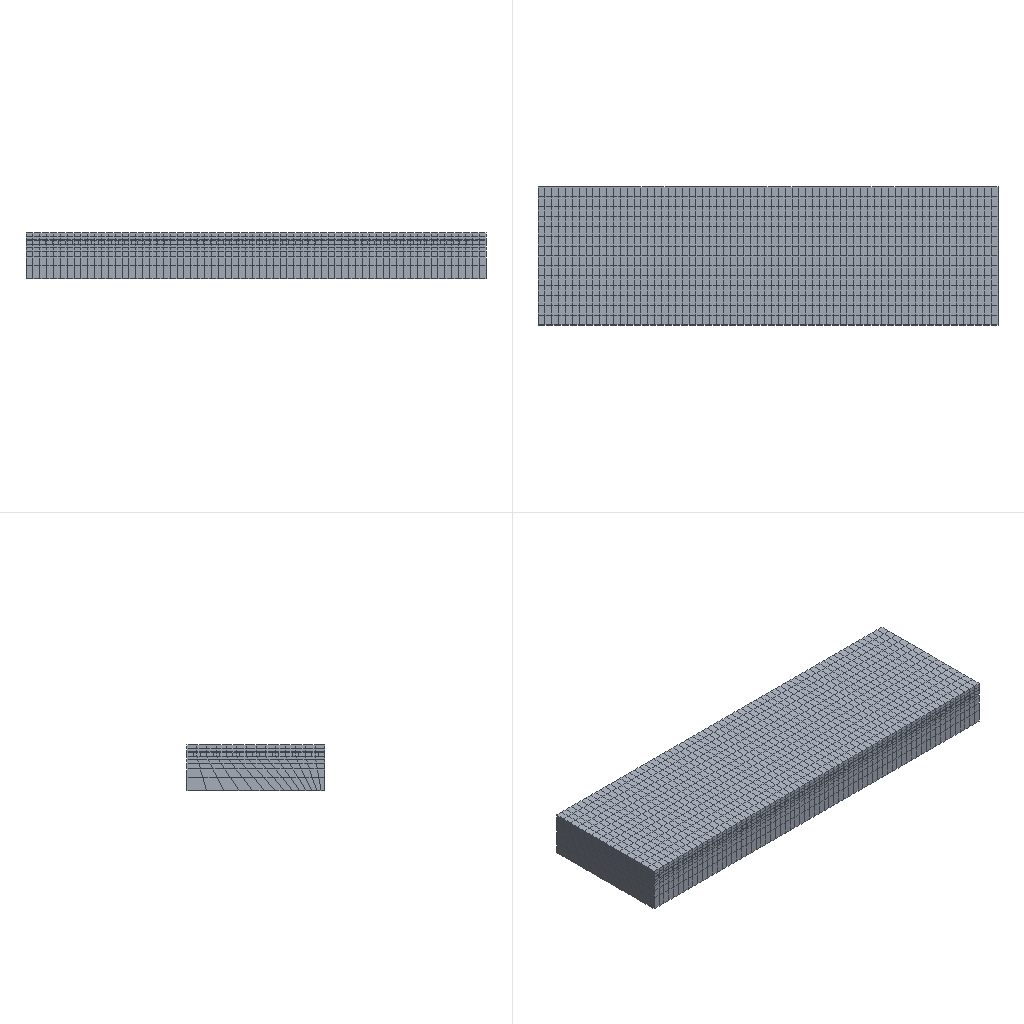Simulation study | abaqus
Set-up summary:
category,name,step,type,value,unit,region
solver,abaqus
solver,version,,,Abaqus/Explicit 2020
units,not stated in the deck,,not stated
analysis,deck,,transient,transient
load_step,Step-1,Step-1,transient
load_step,requested,,,1
mesh,nodes,,,13770
mesh,elements,,,10164
element_type,R3D3,,rigid,228
element_type,R3D4,,rigid,633
element_type,C3D8R,,solid,1470
element_type,COH3D8,,cohesive,329
element_type,EC3D8R,,solid,7504
load,load commands in deck,,count,1
bc,support commands in deck,,count,10
material,BING,,in results
material,COH,,in results
material,WATER,,in results
check,setup vs results,,match,"per instance, exact: element labels, types and connectivity; labels of the nodes the elements use; coordinates of those nodes at SINGLE_PRECISION in 2 of 3 instance(s)"
Abaqus input file, long lists of numbers shortened:
*Heading
** Job name: Job-2 Model name: Model-1-Copy
** Generated by: Abaqus/CAE 2020
*Preprint, echo=NO, model=NO, history=NO, contact=NO
**
** PARTS
**
*Part, name=bing
*Node
      1,        9000.,       -1000.,         900.
      2,        9000.,       -1000.,        1000.
** (3838 more lines like these left out)
*Element, type=C3D8R
 1, 3153, 3154, 1001,  965, 3156, 3155, 3125, 3126
 2,  965, 1001, 1002,  966, 3126, 3125, 3127, 3128
** (1468 more lines like these left out)
*Element, type=COH3D8
1471,  100,   89,    2,    1, 3126, 3125, 3155, 3156
1472,   99,   90,   89,  100, 3128, 3127, 3125, 3126
** (327 more lines like these left out)
*Nset, nset=Set-1
    1,    2,    3,    4,    5,    6,    7,    8,    9,   10,   11,   12,   13,   14,   15,   16
   17,   18,   19,   20,   21,   22,   23,   24,   25,   26,   27,   28,   29,   30,   31,   32
** (238 more lines like these left out)
*Elset, elset=Set-1, generate
    1,  1470,     1
*Elset, elset=CohesiveSeam-1-Elements, generate
 1471,  1799,     1
*Nset, nset=CohesiveSeam-1-TopNodes
 3125, 3126, 3127, 3128, 3129, 3130, 3131, 3132, 3133, 3134, 3135, 3136, 3137, 3138, 3139, 3142
 3143, 3144, 3145, 3146, 3147, 3148, 3149, 3150, 3151, 3152, 3153, 3154, 3155, 3156, 3157, 3158
** (42 more lines like these left out)
*Nset, nset=CohesiveSeam-1-BottomNodes
    1,    2,    3,    4,    5,    8,    9,   10,   11,   12,   13,   14,   17,   18,   19,   20
   21,   22,   23,   24,   25,   26,   27,   28,   29,   30,   31,   32,   33,   34,   35,   36
** (42 more lines like these left out)
*Elset, elset=__PickedSurf21_S1, internal
 1471, 1472, 1473, 1474, 1475, 1476, 1477, 1485, 1486, 1487, 1488, 1489, 1490, 1491, 1506, 1507
 1508, 1509, 1510, 1511, 1512, 1513, 1514, 1515, 1516, 1517, 1518, 1519, 1555, 1556, 1557, 1558
** (5 more lines like these left out)
*Elset, elset=__PickedSurf21_S2, internal
 1478, 1479, 1480, 1481, 1482, 1483, 1484, 1492, 1493, 1494, 1495, 1496, 1497, 1498, 1499, 1500
 1501, 1502, 1503, 1504, 1505, 1520, 1521, 1522, 1523, 1524, 1525, 1526, 1527, 1528, 1529, 1530
** (13 more lines like these left out)
*Surface, type=ELEMENT, name=_PickedSurf21, internal
__PickedSurf21_S1, S1
__PickedSurf21_S2, S2
*Elset, elset=_CohesiveSeam-1-TopSurf_S2, internal, generate
 1471,  1799,     1
*Surface, type=ELEMENT, name=CohesiveSeam-1-TopSurf
_CohesiveSeam-1-TopSurf_S2, S2
*Elset, elset=_CohesiveSeam-1-BottomSurf_S1, internal, generate
 1471,  1799,     1
*Surface, type=ELEMENT, name=CohesiveSeam-1-BottomSurf
_CohesiveSeam-1-BottomSurf_S1, S1
** Section: bing
*Solid Section, elset=Set-1, material=bing
,
** Section: coh
*Cohesive Section, elset=CohesiveSeam-1-Elements, controls=EC-1, material=coh, response=TRACTION SEPARATION
,
*End Part
**
*Part, name=oula
*Node
      1,       10000.,           0.,         750.
      2,       10000.,       -3000.,         750.
** (9178 more lines like these left out)
*Element, type=EC3D8R
   1,  212, 1143, 4033,  615,    1,   13,  511,   46
   2, 1143, 1144, 4034, 4033,   13,   14,  512,  511
** (7502 more lines like these left out)
*Nset, nset=Set-1, generate
    1,  9180,     1
*Elset, elset=Set-1, generate
    1,  7504,     1
** Section: oula
*Eulerian Section, elset=Set-1
water, water-1
*Surface, type=EULERIAN MATERIAL, name=water-1
water-1
*End Part
**
*Part, name=work
*Node
      1,    2.375,   6757.633,   37190.746
      2,    2.375,   6757.633,   40618.258
** (747 more lines like these left out)
*Element, type=R3D4
 1,  1, 21, 64,  4
 2, 21, 22, 63, 64
** (631 more lines like these left out)
*Element, type=R3D3
369,  4, 65,  5
370, 71, 59, 58
** (226 more lines like these left out)
*Node
    750,    2.375,   6959.508,   38910.039
*Nset, nset=work-RefPt_, internal
750,
*Elset, elset=work, generate
   1,  861,    1
*End Part
**
**
** ASSEMBLY
**
*Assembly, name=Assembly
**
*Instance, name=work-1, part=work
37076.822, -1497.625, -5616.383
37076.822, -1497.625, -5616.383, 37077.399, -1498.203, -5616.96,         120.
*End Instance
**
*Instance, name=oula-1, part=oula
          0.,           0.,         250.
*End Instance
**
*Instance, name=bing-1, part=bing
          0.,           0.,         100.
*End Instance
**
*Nset, nset=Set-1, instance=oula-1
    1,    2,    3,    4,    5,    6,    7,    8,   13,   14,   15,   16,   17,   18,   19,   20
   21,   22,   23,   24,   25,   26,   27,   28,   29,   30,   31,   32,   33,   34,   35,   36
** (381 more lines like these left out)
*Elset, elset=Set-1, instance=oula-1, generate
    1,  4690,     1
*Nset, nset=Set-2, instance=bing-1
    5,    6,    7,    8,   13,   14,   15,   16,  101,  102,  103,  104,  105,  106,  107,  108
  109,  110,  111,  112,  149,  150,  151,  152,  153,  154,  155,  156,  157,  158,  159,  160
** (1 more lines like these left out)
*Elset, elset=Set-2, instance=bing-1
  43,  44,  45,  46,  47,  48,  49,  92,  93,  94,  95,  96,  97,  98, 203, 210
 217, 224, 231, 238, 245
*Nset, nset=Set-3, instance=oula-1
    1,    2,    3,    4,    5,    6,    7,    8,    9,   10,   11,   12,   26,   27,   28,   29
   43,   44,   45,   46,   60,   61,   62,   63,   77,   78,   79,   80,   81,   82,   83,   84
** (75 more lines like these left out)
*Elset, elset=Set-3, instance=oula-1
    1,   14,   15,   28,   29,   42,   43,   56,   57,   70,   71,   84,   85,   98,   99,  112
  113,  126,  127,  140,  141,  154,  155,  168,  169,  182,  183,  196,  197,  210,  211,  224
** (65 more lines like these left out)
*Nset, nset=Set-4, instance=oula-1
    3,    4,    6,    7,   30,   31,   32,   33,   34,   35,   36,   37,   38,   39,   40,   41
   42,   64,   65,   66,   67,   68,   69,   70,   71,   72,   73,   74,   75,   76,   81,   82
** (62 more lines like these left out)
*Elset, elset=Set-4, instance=oula-1
   57,   58,   59,   60,   61,   62,   63,   64,   65,   66,   67,   68,   69,   70,  127,  128
  129,  130,  131,  132,  133,  134,  135,  136,  137,  138,  139,  140,  197,  198,  199,  200
** (57 more lines like these left out)
*Nset, nset=Set-5, instance=oula-1
   1,   2,   3,   4,  13,  14,  15,  16,  17,  18,  19,  20,  21,  22,  23,  24
  25,  26,  27,  28,  29,  30,  31,  32,  33,  34,  35,  36,  37,  38,  39,  40
** (4 more lines like these left out)
*Elset, elset=Set-5, instance=oula-1, generate
  1,  70,   1
*Nset, nset=Set-6, instance=work-1
 750,
*Rigid Body, ref node=work-1.work-RefPt_, elset=work-1.work
*End Assembly
**
** ELEMENT CONTROLS
**
*Section Controls, name=EC-1, ELEMENT DELETION=YES
1., 1., 1.
**
** MATERIALS
**
*Material, name=bing
*Brittle Cracking
100.,   0.
250., 0.05
*Brittle Shear
1.,  0.
0., 0.1
*Brittle Failure
 0.01,
*Density
 9.2e-10,
*Elastic
1000., 0.3
*Material, name=coh
*Damage Initiation, criterion=MAXS
10.,10.,10.
*Damage Evolution, type=DISPLACEMENT
 1e-11,
*Density
 9.2e-10,
*Elastic, type=TRACTION
1000.,1000.,1000.
*Material, name=water
*Density
 1e-09,
*Eos, type=USUP
1483.,0.,0.
*Viscosity
 0.01,
**
** INTERACTION PROPERTIES
**
*Surface Interaction, name=IntProp-1
*Friction
 0.2,
*Surface Behavior, pressure-overclosure=HARD
**
** PREDEFINED FIELDS
**
** Name: Predefined Field-1   Type: Material assignment
*Initial Conditions, type=VOLUME FRACTION
Set-1, oula-1.water-1, 1.
** ----------------------------------------------------------------
**
** STEP: Step-1
**
*Step, name=Step-1, nlgeom=YES
*Dynamic, Explicit
, 1.
*Bulk Viscosity
0.06, 1.2
** Mass Scaling: Semi-Automatic
**               Whole Model
*Fixed Mass Scaling, factor=5000.
**
** BOUNDARY CONDITIONS
**
** Name: BC-1 Type: 对称/反对称/完全固定
*Boundary
Set-2, ENCASTRE
** Name: [REDACTED] : Speed/Angular velocity
*Boundary, type=VELOCITY
Set-4, 3, 3
** Name: [REDACTED] : Speed/Angular velocity
*Boundary, type=VELOCITY
Set-5, 1, 1
** Name: [REDACTED] : Speed/Angular velocity
*Boundary, type=VELOCITY
Set-3, 2, 2
** Name: [REDACTED] : Speed/Angular velocity
*Boundary, type=VELOCITY
Set-6, 1, 1, 8300.
Set-6, 2, 2
Set-6, 3, 3
Set-6, 4, 4
Set-6, 5, 5
Set-6, 6, 6
**
** INTERACTIONS
**
** Interaction: Int-1
*Contact, op=NEW
*Contact Inclusions, ALL EXTERIOR
*Contact Property Assignment
 ,  , IntProp-1
**
** OUTPUT REQUESTS
**
*Restart, write, number interval=1, time marks=NO
**
** FIELD OUTPUT: F-Output-1
**
*Output, field, number interval=50
*Node Output
A, CF, RF, RM, RT, U, V
*Element Output, directions=YES
DENSITYVAVG, E, EVF, EVOL, LE, MISES, MISESMAX, PE, PEEQ, PEEQVAVG, PEVAVG, S, SF, SSAVG, STATUS, SVAVG
SVOL, TSHR
*Contact Output
CDISP, CSTRESS
**
** HISTORY OUTPUT: H-Output-1
**
*Output, history, time interval=5e-05
*Node Output, nset=Set-6
RF1, RF2, RF3
*End Step
Results summary:
result,step,Step-1,completed,increments=23872 time=1.0/1.0
result,analysis,,,transient
result,last_loadstep,,,1
result,primary field,,,U
result,reaction total,,FX,-819751.588,model units
result,reaction total,,FY,1195298.288,model units
result,reaction total,,FZ,49678.798,model units